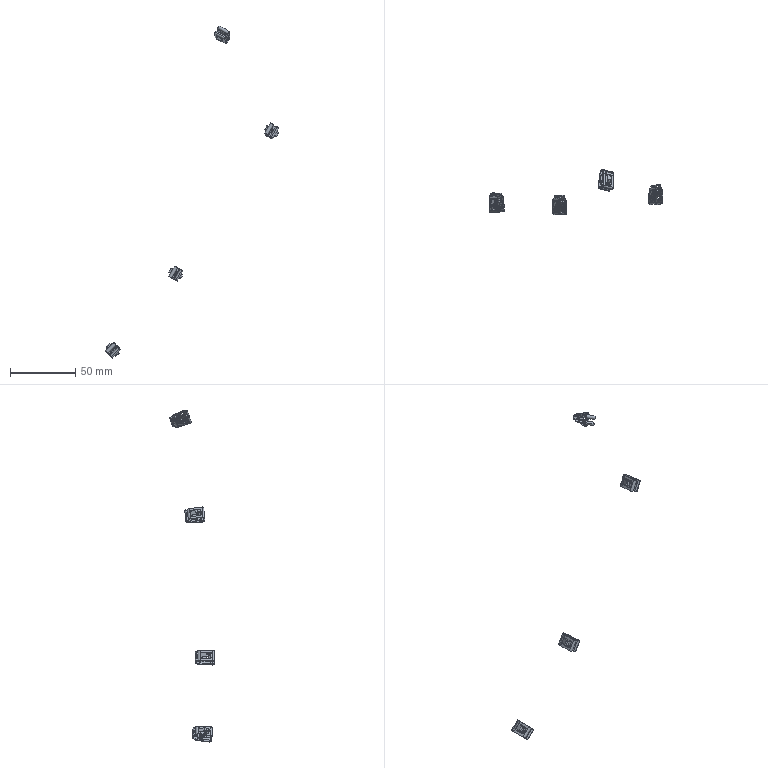Part | SolidWorks | features AEMSimFeature 1 | 4 solids | 1068 faces | box 133.256 x 34.357 x 254.473 mm | volume 678.705 mm3 | plane 492 | cylinder 464 | spline 112 | commonest cylinder face diameters 1 x288 1.8 x72 3 x32 2 x24 1.7 x12 2.5 x12